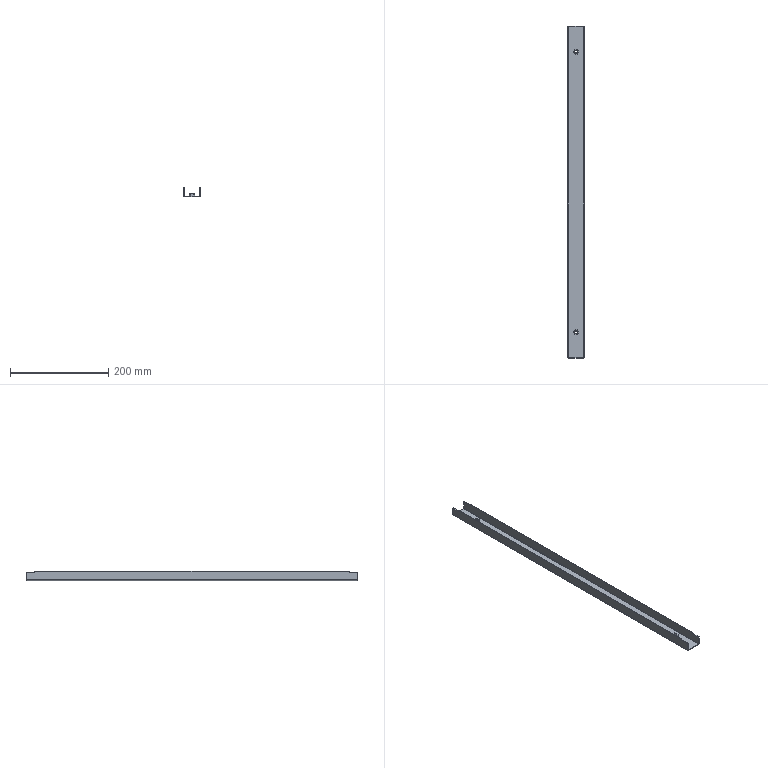Part | SolidWorks | features BaseBody 1 | 1 solid | 54 faces | box 33 x 674.5 x 20 mm | volume 70005 mm3 | plane 42 | cylinder 12 | commonest cylinder face diameters 6 x4 6.5 x4 1 x2 4 x2
STEP:
#1=CARTESIAN_POINT('',(3.,-285.,5.));
#2=VERTEX_POINT('',#1);
#3=CARTESIAN_POINT('',(3.,-285.,0.));
#4=VERTEX_POINT('',#3);
#5=CARTESIAN_POINT('',(3.,-285.,5.));
#6=DIRECTION('',(0.,0.,-1.));
#7=VECTOR('',#6,1000.);
#8=LINE('',#5,#7);
#9=EDGE_CURVE('',#2,#4,#8,.T.);
#10=ORIENTED_EDGE('',*,*,#9,.F.);
#11=CARTESIAN_POINT('',(-3.,-285.,5.));
#12=VERTEX_POINT('',#11);
#13=CARTESIAN_POINT('',(0.,-285.,5.));
#14=DIRECTION('',(0.,0.,1.));
#15=DIRECTION('',(1.,0.,0.));
#16=AXIS2_PLACEMENT_3D('',#13,#14,#15);
#17=CIRCLE('',#16,3.);
#18=EDGE_CURVE('',#2,#12,#17,.T.);
#19=ORIENTED_EDGE('',*,*,#18,.T.);
#20=CARTESIAN_POINT('',(-3.,-285.,0.));
#21=VERTEX_POINT('',#20);
#22=CARTESIAN_POINT('',(-3.,-285.,5.));
#23=DIRECTION('',(0.,0.,-1.));
#24=VECTOR('',#23,1000.);
#25=LINE('',#22,#24);
#26=EDGE_CURVE('',#12,#21,#25,.T.);
#27=ORIENTED_EDGE('',*,*,#26,.T.);
#28=CARTESIAN_POINT('',(0.,-285.,0.));
#29=DIRECTION('',(0.,0.,1.));
#30=DIRECTION('',(1.,0.,0.));
#31=AXIS2_PLACEMENT_3D('',#28,#29,#30);
#32=CIRCLE('',#31,3.);
#33=EDGE_CURVE('',#4,#21,#32,.T.);
#34=ORIENTED_EDGE('',*,*,#33,.F.);
#35=EDGE_LOOP('',(#10,#19,#27,#34));
#36=FACE_OUTER_BOUND('',#35,.T.);
#37=CARTESIAN_POINT('',(0.,-285.,5.));
#38=DIRECTION('',(0.,0.,-1.));
#39=DIRECTION('',(-1.,0.,0.));
#40=AXIS2_PLACEMENT_3D('',#37,#38,#39);
#41=CYLINDRICAL_SURFACE('',#40,3.);
#42=ADVANCED_FACE('',(#36),#41,.F.);
#43=CARTESIAN_POINT('',(3.629,-289.49,0.));
#44=VERTEX_POINT('',#43);
#45=CARTESIAN_POINT('',(5.703,-284.102,0.));
#46=VERTEX_POINT('',#45);
#47=CARTESIAN_POINT('',(3.629,-289.49,0.));
#48=DIRECTION('',(0.3592,0.9333,0.));
#49=VECTOR('',#48,1000.);
#50=LINE('',#47,#49);
#51=EDGE_CURVE('',#44,#46,#50,.T.);
#52=ORIENTED_EDGE('',*,*,#51,.T.);
#53=CARTESIAN_POINT('',(5.703,-284.102,5.));
#54=VERTEX_POINT('',#53);
#55=CARTESIAN_POINT('',(5.703,-284.102,5.));
#56=DIRECTION('',(0.,0.,-1.));
#57=VECTOR('',#56,1000.);
#58=LINE('',#55,#57);
#59=EDGE_CURVE('',#54,#46,#58,.T.);
#60=ORIENTED_EDGE('',*,*,#59,.F.);
#61=CARTESIAN_POINT('',(3.629,-289.49,5.));
#62=VERTEX_POINT('',#61);
#63=CARTESIAN_POINT('',(3.629,-289.49,5.));
#64=DIRECTION('',(0.3592,0.9333,0.));
#65=VECTOR('',#64,1000.);
#66=LINE('',#63,#65);
#67=EDGE_CURVE('',#62,#54,#66,.T.);
#68=ORIENTED_EDGE('',*,*,#67,.F.);
#69=CARTESIAN_POINT('',(3.629,-289.49,5.));
#70=DIRECTION('',(0.,0.,-1.));
#71=VECTOR('',#70,1000.);
#72=LINE('',#69,#71);
#73=EDGE_CURVE('',#62,#44,#72,.T.);
#74=ORIENTED_EDGE('',*,*,#73,.T.);
#75=EDGE_LOOP('',(#52,#60,#68,#74));
#76=FACE_OUTER_BOUND('',#75,.T.);
#77=CARTESIAN_POINT('',(3.629,-289.49,5.));
#78=DIRECTION('',(-0.9333,0.3592,0.));
#79=DIRECTION('',(0.,0.,1.));
#80=AXIS2_PLACEMENT_3D('',#77,#78,#79);
#81=PLANE('',#80);
#82=ADVANCED_FACE('',(#76),#81,.F.);
#83=CARTESIAN_POINT('',(-2.074,-290.388,0.));
#84=VERTEX_POINT('',#83);
#85=CARTESIAN_POINT('',(-2.074,-290.388,0.));
#86=DIRECTION('',(0.9878,0.1555,0.));
#87=VECTOR('',#86,1000.);
#88=LINE('',#85,#87);
#89=EDGE_CURVE('',#84,#44,#88,.T.);
#90=ORIENTED_EDGE('',*,*,#89,.T.);
#91=ORIENTED_EDGE('',*,*,#73,.F.);
#92=CARTESIAN_POINT('',(-2.074,-290.388,5.));
#93=VERTEX_POINT('',#92);
#94=CARTESIAN_POINT('',(-2.074,-290.388,5.));
#95=DIRECTION('',(0.9878,0.1555,0.));
#96=VECTOR('',#95,1000.);
#97=LINE('',#94,#96);
#98=EDGE_CURVE('',#93,#62,#97,.T.);
#99=ORIENTED_EDGE('',*,*,#98,.F.);
#100=CARTESIAN_POINT('',(-2.074,-290.388,5.));
#101=DIRECTION('',(0.,0.,-1.));
#102=VECTOR('',#101,1000.);
#103=LINE('',#100,#102);
#104=EDGE_CURVE('',#93,#84,#103,.T.);
#105=ORIENTED_EDGE('',*,*,#104,.T.);
#106=EDGE_LOOP('',(#90,#91,#99,#105));
#107=FACE_OUTER_BOUND('',#106,.T.);
#108=CARTESIAN_POINT('',(-2.074,-290.388,5.));
#109=DIRECTION('',(-0.1555,0.9878,0.));
#110=DIRECTION('',(0.,0.,1.));
#111=AXIS2_PLACEMENT_3D('',#108,#109,#110);
#112=PLANE('',#111);
#113=ADVANCED_FACE('',(#107),#112,.F.);
#114=CARTESIAN_POINT('',(-5.703,-285.898,0.));
#115=VERTEX_POINT('',#114);
#116=CARTESIAN_POINT('',(-5.703,-285.898,0.));
#117=DIRECTION('',(0.6286,-0.7777,0.));
#118=VECTOR('',#117,1000.);
#119=LINE('',#116,#118);
#120=EDGE_CURVE('',#115,#84,#119,.T.);
#121=ORIENTED_EDGE('',*,*,#120,.T.);
#122=ORIENTED_EDGE('',*,*,#104,.F.);
#123=CARTESIAN_POINT('',(-5.703,-285.898,5.));
#124=VERTEX_POINT('',#123);
#125=CARTESIAN_POINT('',(-5.703,-285.898,5.));
#126=DIRECTION('',(0.6286,-0.7777,0.));
#127=VECTOR('',#126,1000.);
#128=LINE('',#125,#127);
#129=EDGE_CURVE('',#124,#93,#128,.T.);
#130=ORIENTED_EDGE('',*,*,#129,.F.);
#131=CARTESIAN_POINT('',(-5.703,-285.898,5.));
#132=DIRECTION('',(0.,0.,-1.));
#133=VECTOR('',#132,1000.);
#134=LINE('',#131,#133);
#135=EDGE_CURVE('',#124,#115,#134,.T.);
#136=ORIENTED_EDGE('',*,*,#135,.T.);
#137=EDGE_LOOP('',(#121,#122,#130,#136));
#138=FACE_OUTER_BOUND('',#137,.T.);
#139=CARTESIAN_POINT('',(-5.703,-285.898,5.));
#140=DIRECTION('',(0.7777,0.6286,0.));
#141=DIRECTION('',(0.,0.,-1.));
#142=AXIS2_PLACEMENT_3D('',#139,#140,#141);
#143=PLANE('',#142);
#144=ADVANCED_FACE('',(#138),#143,.F.);
#145=CARTESIAN_POINT('',(-3.629,-280.51,0.));
#146=VERTEX_POINT('',#145);
#147=CARTESIAN_POINT('',(-3.629,-280.51,0.));
#148=DIRECTION('',(-0.3592,-0.9333,0.));
#149=VECTOR('',#148,1000.);
#150=LINE('',#147,#149);
#151=EDGE_CURVE('',#146,#115,#150,.T.);
#152=ORIENTED_EDGE('',*,*,#151,.T.);
#153=ORIENTED_EDGE('',*,*,#135,.F.);
#154=CARTESIAN_POINT('',(-3.629,-280.51,5.));
#155=VERTEX_POINT('',#154);
#156=CARTESIAN_POINT('',(-3.629,-280.51,5.));
#157=DIRECTION('',(-0.3592,-0.9333,0.));
#158=VECTOR('',#157,1000.);
#159=LINE('',#156,#158);
#160=EDGE_CURVE('',#155,#124,#159,.T.);
#161=ORIENTED_EDGE('',*,*,#160,.F.);
#162=CARTESIAN_POINT('',(-3.629,-280.51,5.));
#163=DIRECTION('',(0.,0.,-1.));
#164=VECTOR('',#163,1000.);
#165=LINE('',#162,#164);
#166=EDGE_CURVE('',#155,#146,#165,.T.);
#167=ORIENTED_EDGE('',*,*,#166,.T.);
#168=EDGE_LOOP('',(#152,#153,#161,#167));
#169=FACE_OUTER_BOUND('',#168,.T.);
#170=CARTESIAN_POINT('',(-3.629,-280.51,5.));
#171=DIRECTION('',(0.9333,-0.3592,0.));
#172=DIRECTION('',(0.,0.,-1.));
#173=AXIS2_PLACEMENT_3D('',#170,#171,#172);
#174=PLANE('',#173);
#175=ADVANCED_FACE('',(#169),#174,.F.);
#176=CARTESIAN_POINT('',(2.074,-279.612,0.));
#177=VERTEX_POINT('',#176);
#178=CARTESIAN_POINT('',(2.074,-279.612,0.));
#179=DIRECTION('',(-0.9878,-0.1555,0.));
#180=VECTOR('',#179,1000.);
#181=LINE('',#178,#180);
#182=EDGE_CURVE('',#177,#146,#181,.T.);
#183=ORIENTED_EDGE('',*,*,#182,.T.);
#184=ORIENTED_EDGE('',*,*,#166,.F.);
#185=CARTESIAN_POINT('',(2.074,-279.612,5.));
#186=VERTEX_POINT('',#185);
#187=CARTESIAN_POINT('',(2.074,-279.612,5.));
#188=DIRECTION('',(-0.9878,-0.1555,0.));
#189=VECTOR('',#188,1000.);
#190=LINE('',#187,#189);
#191=EDGE_CURVE('',#186,#155,#190,.T.);
#192=ORIENTED_EDGE('',*,*,#191,.F.);
#193=CARTESIAN_POINT('',(2.074,-279.612,5.));
#194=DIRECTION('',(0.,0.,-1.));
#195=VECTOR('',#194,1000.);
#196=LINE('',#193,#195);
#197=EDGE_CURVE('',#186,#177,#196,.T.);
#198=ORIENTED_EDGE('',*,*,#197,.T.);
#199=EDGE_LOOP('',(#183,#184,#192,#198));
#200=FACE_OUTER_BOUND('',#199,.T.);
#201=CARTESIAN_POINT('',(2.074,-279.612,5.));
#202=DIRECTION('',(0.1555,-0.9878,0.));
#203=DIRECTION('',(0.,0.,-1.));
#204=AXIS2_PLACEMENT_3D('',#201,#202,#203);
#205=PLANE('',#204);
#206=ADVANCED_FACE('',(#200),#205,.F.);
#207=CARTESIAN_POINT('',(5.703,-284.102,0.));
#208=DIRECTION('',(-0.6286,0.7777,0.));
#209=VECTOR('',#208,1000.);
#210=LINE('',#207,#209);
#211=EDGE_CURVE('',#46,#177,#210,.T.);
#212=ORIENTED_EDGE('',*,*,#211,.T.);
#213=ORIENTED_EDGE('',*,*,#197,.F.);
#214=CARTESIAN_POINT('',(5.703,-284.102,5.));
#215=DIRECTION('',(-0.6286,0.7777,0.));
#216=VECTOR('',#215,1000.);
#217=LINE('',#214,#216);
#218=EDGE_CURVE('',#54,#186,#217,.T.);
#219=ORIENTED_EDGE('',*,*,#218,.F.);
#220=ORIENTED_EDGE('',*,*,#59,.T.);
#221=EDGE_LOOP('',(#212,#213,#219,#220));
#222=FACE_OUTER_BOUND('',#221,.T.);
#223=CARTESIAN_POINT('',(5.703,-284.102,5.));
#224=DIRECTION('',(-0.7777,-0.6286,0.));
#225=DIRECTION('',(-0.6286,0.7777,0.));
#226=AXIS2_PLACEMENT_3D('',#223,#224,#225);
#227=PLANE('',#226);
#228=ADVANCED_FACE('',(#222),#227,.F.);
#229=CARTESIAN_POINT('',(0.,-285.,5.));
#230=DIRECTION('',(0.,0.,1.));
#231=DIRECTION('',(1.,0.,0.));
#232=AXIS2_PLACEMENT_3D('',#229,#230,#231);
#233=CIRCLE('',#232,3.);
#234=EDGE_CURVE('',#12,#2,#233,.T.);
#235=ORIENTED_EDGE('',*,*,#234,.F.);
#236=ORIENTED_EDGE('',*,*,#18,.F.);
#237=EDGE_LOOP('',(#235,#236));
#238=FACE_BOUND('',#237,.T.);
#239=ORIENTED_EDGE('',*,*,#218,.T.);
#240=ORIENTED_EDGE('',*,*,#191,.T.);
#241=ORIENTED_EDGE('',*,*,#160,.T.);
#242=ORIENTED_EDGE('',*,*,#129,.T.);
#243=ORIENTED_EDGE('',*,*,#98,.T.);
#244=ORIENTED_EDGE('',*,*,#67,.T.);
#245=EDGE_LOOP('',(#239,#240,#241,#242,#243,#244));
#246=FACE_OUTER_BOUND('',#245,.T.);
#247=CARTESIAN_POINT('',(0.,0.,5.));
#248=DIRECTION('',(0.,0.,1.));
#249=DIRECTION('',(1.,0.,0.));
#250=AXIS2_PLACEMENT_3D('',#247,#248,#249);
#251=PLANE('',#250);
#252=ADVANCED_FACE('',(#238,#246),#251,.T.);
#253=CARTESIAN_POINT('',(0.,-285.,0.));
#254=DIRECTION('',(0.,0.,1.));
#255=DIRECTION('',(1.,0.,0.));
#256=AXIS2_PLACEMENT_3D('',#253,#254,#255);
#257=CIRCLE('',#256,3.);
#258=EDGE_CURVE('',#21,#4,#257,.T.);
#259=ORIENTED_EDGE('',*,*,#258,.T.);
#260=ORIENTED_EDGE('',*,*,#33,.T.);
#261=EDGE_LOOP('',(#259,#260));
#262=FACE_BOUND('',#261,.T.);
#263=CARTESIAN_POINT('',(-3.25,-285.,0.));
#264=VERTEX_POINT('',#263);
#265=CARTESIAN_POINT('',(3.25,-285.,0.));
#266=VERTEX_POINT('',#265);
#267=CARTESIAN_POINT('',(0.,-285.,0.));
#268=DIRECTION('',(0.,0.,-1.));
#269=DIRECTION('',(-1.,0.,0.));
#270=AXIS2_PLACEMENT_3D('',#267,#268,#269);
#271=CIRCLE('',#270,3.25);
#272=EDGE_CURVE('',#264,#266,#271,.T.);
#273=ORIENTED_EDGE('',*,*,#272,.T.);
#274=CARTESIAN_POINT('',(0.,-285.,0.));
#275=DIRECTION('',(0.,0.,-1.));
#276=DIRECTION('',(-1.,0.,0.));
#277=AXIS2_PLACEMENT_3D('',#274,#275,#276);
#278=CIRCLE('',#277,3.25);
#279=EDGE_CURVE('',#266,#264,#278,.T.);
#280=ORIENTED_EDGE('',*,*,#279,.T.);
#281=EDGE_LOOP('',(#273,#280));
#282=FACE_OUTER_BOUND('',#281,.T.);
#283=CARTESIAN_POINT('',(0.,0.,0.));
#284=DIRECTION('',(0.,0.,1.));
#285=DIRECTION('',(1.,0.,0.));
#286=AXIS2_PLACEMENT_3D('',#283,#284,#285);
#287=PLANE('',#286);
#288=ADVANCED_FACE('',(#262,#282),#287,.F.);
#289=CARTESIAN_POINT('',(3.,285.,5.));
#290=VERTEX_POINT('',#289);
#291=CARTESIAN_POINT('',(3.,285.,0.));
#292=VERTEX_POINT('',#291);
#293=CARTESIAN_POINT('',(3.,285.,5.));
#294=DIRECTION('',(0.,0.,-1.));
#295=VECTOR('',#294,1000.);
#296=LINE('',#293,#295);
#297=EDGE_CURVE('',#290,#292,#296,.T.);
#298=ORIENTED_EDGE('',*,*,#297,.F.);
#299=CARTESIAN_POINT('',(-3.,285.,5.));
#300=VERTEX_POINT('',#299);
#301=CARTESIAN_POINT('',(0.,285.,5.));
#302=DIRECTION('',(0.,0.,1.));
#303=DIRECTION('',(1.,0.,0.));
#304=AXIS2_PLACEMENT_3D('',#301,#302,#303);
#305=CIRCLE('',#304,3.);
#306=EDGE_CURVE('',#290,#300,#305,.T.);
#307=ORIENTED_EDGE('',*,*,#306,.T.);
#308=CARTESIAN_POINT('',(-3.,285.,0.));
#309=VERTEX_POINT('',#308);
#310=CARTESIAN_POINT('',(-3.,285.,5.));
#311=DIRECTION('',(0.,0.,-1.));
#312=VECTOR('',#311,1000.);
#313=LINE('',#310,#312);
#314=EDGE_CURVE('',#300,#309,#313,.T.);
#315=ORIENTED_EDGE('',*,*,#314,.T.);
#316=CARTESIAN_POINT('',(0.,285.,0.));
#317=DIRECTION('',(0.,0.,1.));
#318=DIRECTION('',(1.,0.,0.));
#319=AXIS2_PLACEMENT_3D('',#316,#317,#318);
#320=CIRCLE('',#319,3.);
#321=EDGE_CURVE('',#292,#309,#320,.T.);
#322=ORIENTED_EDGE('',*,*,#321,.F.);
#323=EDGE_LOOP('',(#298,#307,#315,#322));
#324=FACE_OUTER_BOUND('',#323,.T.);
#325=CARTESIAN_POINT('',(0.,285.,5.));
#326=DIRECTION('',(0.,0.,-1.));
#327=DIRECTION('',(-1.,0.,0.));
#328=AXIS2_PLACEMENT_3D('',#325,#326,#327);
#329=CYLINDRICAL_SURFACE('',#328,3.);
#330=ADVANCED_FACE('',(#324),#329,.F.);
#331=CARTESIAN_POINT('',(-5.703,285.898,0.));
#332=VERTEX_POINT('',#331);
#333=CARTESIAN_POINT('',(-3.629,280.51,0.));
#334=VERTEX_POINT('',#333);
#335=CARTESIAN_POINT('',(-5.703,285.898,0.));
#336=DIRECTION('',(0.3592,-0.9333,0.));
#337=VECTOR('',#336,1000.);
#338=LINE('',#335,#337);
#339=EDGE_CURVE('',#332,#334,#338,.T.);
#340=ORIENTED_EDGE('',*,*,#339,.T.);
#341=CARTESIAN_POINT('',(-3.629,280.51,5.));
#342=VERTEX_POINT('',#341);
#343=CARTESIAN_POINT('',(-3.629,280.51,5.));
#344=DIRECTION('',(0.,0.,-1.));
#345=VECTOR('',#344,1000.);
#346=LINE('',#343,#345);
#347=EDGE_CURVE('',#342,#334,#346,.T.);
#348=ORIENTED_EDGE('',*,*,#347,.F.);
#349=CARTESIAN_POINT('',(-5.703,285.898,5.));
#350=VERTEX_POINT('',#349);
#351=CARTESIAN_POINT('',(-5.703,285.898,5.));
#352=DIRECTION('',(0.3592,-0.9333,0.));
#353=VECTOR('',#352,1000.);
#354=LINE('',#351,#353);
#355=EDGE_CURVE('',#350,#342,#354,.T.);
#356=ORIENTED_EDGE('',*,*,#355,.F.);
#357=CARTESIAN_POINT('',(-5.703,285.898,5.));
#358=DIRECTION('',(0.,0.,-1.));
#359=VECTOR('',#358,1000.);
#360=LINE('',#357,#359);
#361=EDGE_CURVE('',#350,#332,#360,.T.);
#362=ORIENTED_EDGE('',*,*,#361,.T.);
#363=EDGE_LOOP('',(#340,#348,#356,#362));
#364=FACE_OUTER_BOUND('',#363,.T.);
#365=CARTESIAN_POINT('',(-5.703,285.898,5.));
#366=DIRECTION('',(0.9333,0.3592,0.));
#367=DIRECTION('',(0.,0.,-1.));
#368=AXIS2_PLACEMENT_3D('',#365,#366,#367);
#369=PLANE('',#368);
#370=ADVANCED_FACE('',(#364),#369,.F.);
#371=CARTESIAN_POINT('',(-2.074,290.388,0.));
#372=VERTEX_POINT('',#371);
#373=CARTESIAN_POINT('',(-2.074,290.388,0.));
#374=DIRECTION('',(-0.6286,-0.7777,0.));
#375=VECTOR('',#374,1000.);
#376=LINE('',#373,#375);
#377=EDGE_CURVE('',#372,#332,#376,.T.);
#378=ORIENTED_EDGE('',*,*,#377,.T.);
#379=ORIENTED_EDGE('',*,*,#361,.F.);
#380=CARTESIAN_POINT('',(-2.074,290.388,5.));
#381=VERTEX_POINT('',#380);
#382=CARTESIAN_POINT('',(-2.074,290.388,5.));
#383=DIRECTION('',(-0.6286,-0.7777,0.));
#384=VECTOR('',#383,1000.);
#385=LINE('',#382,#384);
#386=EDGE_CURVE('',#381,#350,#385,.T.);
#387=ORIENTED_EDGE('',*,*,#386,.F.);
#388=CARTESIAN_POINT('',(-2.074,290.388,5.));
#389=DIRECTION('',(0.,0.,-1.));
#390=VECTOR('',#389,1000.);
#391=LINE('',#388,#390);
#392=EDGE_CURVE('',#381,#372,#391,.T.);
#393=ORIENTED_EDGE('',*,*,#392,.T.);
#394=EDGE_LOOP('',(#378,#379,#387,#393));
#395=FACE_OUTER_BOUND('',#394,.T.);
#396=CARTESIAN_POINT('',(-2.074,290.388,5.));
#397=DIRECTION('',(0.7777,-0.6286,0.));
#398=DIRECTION('',(0.,0.,-1.));
#399=AXIS2_PLACEMENT_3D('',#396,#397,#398);
#400=PLANE('',#399);
#401=ADVANCED_FACE('',(#395),#400,.F.);
#402=CARTESIAN_POINT('',(3.629,289.49,0.));
#403=VERTEX_POINT('',#402);
#404=CARTESIAN_POINT('',(3.629,289.49,0.));
#405=DIRECTION('',(-0.9878,0.1555,0.));
#406=VECTOR('',#405,1000.);
#407=LINE('',#404,#406);
#408=EDGE_CURVE('',#403,#372,#407,.T.);
#409=ORIENTED_EDGE('',*,*,#408,.T.);
#410=ORIENTED_EDGE('',*,*,#392,.F.);
#411=CARTESIAN_POINT('',(3.629,289.49,5.));
#412=VERTEX_POINT('',#411);
#413=CARTESIAN_POINT('',(3.629,289.49,5.));
#414=DIRECTION('',(-0.9878,0.1555,0.));
#415=VECTOR('',#414,1000.);
#416=LINE('',#413,#415);
#417=EDGE_CURVE('',#412,#381,#416,.T.);
#418=ORIENTED_EDGE('',*,*,#417,.F.);
#419=CARTESIAN_POINT('',(3.629,289.49,5.));
#420=DIRECTION('',(0.,0.,-1.));
#421=VECTOR('',#420,1000.);
#422=LINE('',#419,#421);
#423=EDGE_CURVE('',#412,#403,#422,.T.);
#424=ORIENTED_EDGE('',*,*,#423,.T.);
#425=EDGE_LOOP('',(#409,#410,#418,#424));
#426=FACE_OUTER_BOUND('',#425,.T.);
#427=CARTESIAN_POINT('',(3.629,289.49,5.));
#428=DIRECTION('',(-0.1555,-0.9878,0.));
#429=DIRECTION('',(-0.9878,0.1555,0.));
#430=AXIS2_PLACEMENT_3D('',#427,#428,#429);
#431=PLANE('',#430);
#432=ADVANCED_FACE('',(#426),#431,.F.);
#433=CARTESIAN_POINT('',(5.703,284.102,0.));
#434=VERTEX_POINT('',#433);
#435=CARTESIAN_POINT('',(5.703,284.102,0.));
#436=DIRECTION('',(-0.3592,0.9333,0.));
#437=VECTOR('',#436,1000.);
#438=LINE('',#435,#437);
#439=EDGE_CURVE('',#434,#403,#438,.T.);
#440=ORIENTED_EDGE('',*,*,#439,.T.);
#441=ORIENTED_EDGE('',*,*,#423,.F.);
#442=CARTESIAN_POINT('',(5.703,284.102,5.));
#443=VERTEX_POINT('',#442);
#444=CARTESIAN_POINT('',(5.703,284.102,5.));
#445=DIRECTION('',(-0.3592,0.9333,0.));
#446=VECTOR('',#445,1000.);
#447=LINE('',#444,#446);
#448=EDGE_CURVE('',#443,#412,#447,.T.);
#449=ORIENTED_EDGE('',*,*,#448,.F.);
#450=CARTESIAN_POINT('',(5.703,284.102,5.));
#451=DIRECTION('',(0.,0.,-1.));
#452=VECTOR('',#451,1000.);
#453=LINE('',#450,#452);
#454=EDGE_CURVE('',#443,#434,#453,.T.);
#455=ORIENTED_EDGE('',*,*,#454,.T.);
#456=EDGE_LOOP('',(#440,#441,#449,#455));
#457=FACE_OUTER_BOUND('',#456,.T.);
#458=CARTESIAN_POINT('',(5.703,284.102,5.));
#459=DIRECTION('',(-0.9333,-0.3592,0.));
#460=DIRECTION('',(-0.3592,0.9333,0.));
#461=AXIS2_PLACEMENT_3D('',#458,#459,#460);
#462=PLANE('',#461);
#463=ADVANCED_FACE('',(#457),#462,.F.);
#464=CARTESIAN_POINT('',(2.074,279.612,0.));
#465=VERTEX_POINT('',#464);
#466=CARTESIAN_POINT('',(2.074,279.612,0.));
#467=DIRECTION('',(0.6286,0.7777,0.));
#468=VECTOR('',#467,1000.);
#469=LINE('',#466,#468);
#470=EDGE_CURVE('',#465,#434,#469,.T.);
#471=ORIENTED_EDGE('',*,*,#470,.T.);
#472=ORIENTED_EDGE('',*,*,#454,.F.);
#473=CARTESIAN_POINT('',(2.074,279.612,5.));
#474=VERTEX_POINT('',#473);
#475=CARTESIAN_POINT('',(2.074,279.612,5.));
#476=DIRECTION('',(0.6286,0.7777,0.));
#477=VECTOR('',#476,1000.);
#478=LINE('',#475,#477);
#479=EDGE_CURVE('',#474,#443,#478,.T.);
#480=ORIENTED_EDGE('',*,*,#479,.F.);
#481=CARTESIAN_POINT('',(2.074,279.612,5.));
#482=DIRECTION('',(0.,0.,-1.));
#483=VECTOR('',#482,1000.);
#484=LINE('',#481,#483);
#485=EDGE_CURVE('',#474,#465,#484,.T.);
#486=ORIENTED_EDGE('',*,*,#485,.T.);
#487=EDGE_LOOP('',(#471,#472,#480,#486));
#488=FACE_OUTER_BOUND('',#487,.T.);
#489=CARTESIAN_POINT('',(2.074,279.612,5.));
#490=DIRECTION('',(-0.7777,0.6286,0.));
#491=DIRECTION('',(0.,0.,1.));
#492=AXIS2_PLACEMENT_3D('',#489,#490,#491);
#493=PLANE('',#492);
#494=ADVANCED_FACE('',(#488),#493,.F.);
#495=CARTESIAN_POINT('',(-3.629,280.51,0.));
#496=DIRECTION('',(0.9878,-0.1555,0.));
#497=VECTOR('',#496,1000.);
#498=LINE('',#495,#497);
#499=EDGE_CURVE('',#334,#465,#498,.T.);
#500=ORIENTED_EDGE('',*,*,#499,.T.);
#501=ORIENTED_EDGE('',*,*,#485,.F.);
#502=CARTESIAN_POINT('',(-3.629,280.51,5.));
#503=DIRECTION('',(0.9878,-0.1555,0.));
#504=VECTOR('',#503,1000.);
#505=LINE('',#502,#504);
#506=EDGE_CURVE('',#342,#474,#505,.T.);
#507=ORIENTED_EDGE('',*,*,#506,.F.);
#508=ORIENTED_EDGE('',*,*,#347,.T.);
#509=EDGE_LOOP('',(#500,#501,#507,#508));
#510=FACE_OUTER_BOUND('',#509,.T.);
#511=CARTESIAN_POINT('',(-3.629,280.51,5.));
#512=DIRECTION('',(0.1555,0.9878,0.));
#513=DIRECTION('',(0.,0.,-1.));
#514=AXIS2_PLACEMENT_3D('',#511,#512,#513);
#515=PLANE('',#514);
#516=ADVANCED_FACE('',(#510),#515,.F.);
#517=CARTESIAN_POINT('',(0.,285.,5.));
#518=DIRECTION('',(0.,0.,1.));
#519=DIRECTION('',(1.,0.,0.));
#520=AXIS2_PLACEMENT_3D('',#517,#518,#519);
#521=CIRCLE('',#520,3.);
#522=EDGE_CURVE('',#300,#290,#521,.T.);
#523=ORIENTED_EDGE('',*,*,#522,.F.);
#524=ORIENTED_EDGE('',*,*,#306,.F.);
#525=EDGE_LOOP('',(#523,#524));
#526=FACE_BOUND('',#525,.T.);
#527=ORIENTED_EDGE('',*,*,#506,.T.);
#528=ORIENTED_EDGE('',*,*,#479,.T.);
#529=ORIENTED_EDGE('',*,*,#448,.T.);
#530=ORIENTED_EDGE('',*,*,#417,.T.);
#531=ORIENTED_EDGE('',*,*,#386,.T.);
#532=ORIENTED_EDGE('',*,*,#355,.T.);
#533=EDGE_LOOP('',(#527,#528,#529,#530,#531,#532));
#534=FACE_OUTER_BOUND('',#533,.T.);
#535=CARTESIAN_POINT('',(0.,0.,5.));
#536=DIRECTION('',(0.,0.,1.));
#537=DIRECTION('',(1.,0.,0.));
#538=AXIS2_PLACEMENT_3D('',#535,#536,#537);
#539=PLANE('',#538);
#540=ADVANCED_FACE('',(#526,#534),#539,.T.);
#541=CARTESIAN_POINT('',(0.,285.,0.));
#542=DIRECTION('',(0.,0.,1.));
#543=DIRECTION('',(1.,0.,0.));
#544=AXIS2_PLACEMENT_3D('',#541,#542,#543);
#545=CIRCLE('',#544,3.);
#546=EDGE_CURVE('',#309,#292,#545,.T.);
#547=ORIENTED_EDGE('',*,*,#546,.T.);
#548=ORIENTED_EDGE('',*,*,#321,.T.);
#549=EDGE_LOOP('',(#547,#548));
#550=FACE_BOUND('',#549,.T.);
#551=CARTESIAN_POINT('',(-3.25,285.,0.));
#552=VERTEX_POINT('',#551);
#553=CARTESIAN_POINT('',(3.25,285.,0.));
#554=VERTEX_POINT('',#553);
#555=CARTESIAN_POINT('',(0.,285.,0.));
#556=DIRECTION('',(0.,0.,-1.));
#557=DIRECTION('',(-1.,0.,0.));
#558=AXIS2_PLACEMENT_3D('',#555,#556,#557);
#559=CIRCLE('',#558,3.25);
#560=EDGE_CURVE('',#552,#554,#559,.T.);
#561=ORIENTED_EDGE('',*,*,#560,.T.);
#562=CARTESIAN_POINT('',(0.,285.,0.));
#563=DIRECTION('',(0.,0.,-1.));
#564=DIRECTION('',(-1.,0.,0.));
#565=AXIS2_PLACEMENT_3D('',#562,#563,#564);
#566=CIRCLE('',#565,3.25);
#567=EDGE_CURVE('',#554,#552,#566,.T.);
#568=ORIENTED_EDGE('',*,*,#567,.T.);
#569=EDGE_LOOP('',(#561,#568));
#570=FACE_OUTER_BOUND('',#569,.T.);
#571=CARTESIAN_POINT('',(0.,0.,0.));
#572=DIRECTION('',(0.,0.,1.));
#573=DIRECTION('',(1.,0.,0.));
#574=AXIS2_PLACEMENT_3D('',#571,#572,#573);
#575=PLANE('',#574);
#576=ADVANCED_FACE('',(#550,#570),#575,.F.);
#577=CARTESIAN_POINT('',(-15.,319.25,18.5));
#578=VERTEX_POINT('',#577);
#579=CARTESIAN_POINT('',(-15.,319.25,16.5));
#580=VERTEX_POINT('',#579);
#581=CARTESIAN_POINT('',(-15.,319.25,0.));
#582=DIRECTION('',(0.,0.,-1.));
#583=VECTOR('',#582,1000.);
#584=LINE('',#581,#583);
#585=EDGE_CURVE('',#578,#580,#584,.T.);
#586=ORIENTED_EDGE('',*,*,#585,.T.);
#587=CARTESIAN_POINT('',(-16.5,319.25,16.5));
#588=VERTEX_POINT('',#587);
#589=CARTESIAN_POINT('',(-16.5,319.25,16.5));
#590=DIRECTION('',(1.,0.,0.));
#591=VECTOR('',#590,1000.);
#592=LINE('',#589,#591);
#593=EDGE_CURVE('',#588,#580,#592,.T.);
#594=ORIENTED_EDGE('',*,*,#593,.F.);
#595=CARTESIAN_POINT('',(-16.5,319.25,18.5));
#596=VERTEX_POINT('',#595);
#597=CARTESIAN_POINT('',(-16.5,319.25,18.5));
#598=DIRECTION('',(0.,0.,-1.));
#599=VECTOR('',#598,1000.);
#600=LINE('',#597,#599);
#601=EDGE_CURVE('',#596,#588,#600,.T.);
#602=ORIENTED_EDGE('',*,*,#601,.F.);
#603=CARTESIAN_POINT('',(-16.5,319.25,18.5));
#604=DIRECTION('',(1.,0.,0.));
#605=VECTOR('',#604,1000.);
#606=LINE('',#603,#605);
#607=EDGE_CURVE('',#596,#578,#606,.T.);
#608=ORIENTED_EDGE('',*,*,#607,.T.);
#609=EDGE_LOOP('',(#586,#594,#602,#608));
#610=FACE_OUTER_BOUND('',#609,.T.);
#611=CARTESIAN_POINT('',(-16.5,319.25,18.5));
#612=DIRECTION('',(0.,-1.,0.));
#613=DIRECTION('',(0.,0.,-1.));
#614=AXIS2_PLACEMENT_3D('',#611,#612,#613);
#615=PLANE('',#614);
#616=ADVANCED_FACE('',(#610),#615,.F.);
#617=CARTESIAN_POINT('',(-15.,337.25,16.5));
#618=VERTEX_POINT('',#617);
#619=CARTESIAN_POINT('',(-15.,0.,16.5));
#620=DIRECTION('',(0.,1.,0.));
#621=VECTOR('',#620,1000.);
#622=LINE('',#619,#621);
#623=EDGE_CURVE('',#580,#618,#622,.T.);
#624=ORIENTED_EDGE('',*,*,#623,.T.);
#625=CARTESIAN_POINT('',(-16.5,337.25,16.5));
#626=VERTEX_POINT('',#625);
#627=CARTESIAN_POINT('',(-16.5,337.25,16.5));
#628=DIRECTION('',(1.,0.,0.));
#629=VECTOR('',#628,1000.);
#630=LINE('',#627,#629);
#631=EDGE_CURVE('',#626,#618,#630,.T.);
#632=ORIENTED_EDGE('',*,*,#631,.F.);
#633=CARTESIAN_POINT('',(-16.5,337.25,16.5));
#634=DIRECTION('',(0.,1.,0.));
#635=VECTOR('',#634,1000.);
#636=LINE('',#633,#635);
#637=EDGE_CURVE('',#588,#626,#636,.T.);
#638=ORIENTED_EDGE('',*,*,#637,.F.);
#639=ORIENTED_EDGE('',*,*,#593,.T.);
#640=EDGE_LOOP('',(#624,#632,#638,#639));
#641=FACE_OUTER_BOUND('',#640,.T.);
#642=CARTESIAN_POINT('',(-16.5,337.25,16.5));
#643=DIRECTION('',(0.,0.,-1.));
#644=DIRECTION('',(-1.,0.,0.));
#645=AXIS2_PLACEMENT_3D('',#642,#643,#644);
#646=PLANE('',#645);
#647=ADVANCED_FACE('',(#641),#646,.F.);
#648=CARTESIAN_POINT('',(-15.,-319.25,16.5));
#649=VERTEX_POINT('',#648);
#650=CARTESIAN_POINT('',(-15.,-319.25,18.5));
#651=VERTEX_POINT('',#650);
#652=CARTESIAN_POINT('',(-15.,-319.25,0.));
#653=DIRECTION('',(0.,0.,1.));
#654=VECTOR('',#653,1000.);
#655=LINE('',#652,#654);
#656=EDGE_CURVE('',#649,#651,#655,.T.);
#657=ORIENTED_EDGE('',*,*,#656,.T.);
#658=CARTESIAN_POINT('',(-16.5,-319.25,18.5));
#659=VERTEX_POINT('',#658);
#660=CARTESIAN_POINT('',(-16.5,-319.25,18.5));
#661=DIRECTION('',(1.,0.,0.));
#662=VECTOR('',#661,1000.);
#663=LINE('',#660,#662);
#664=EDGE_CURVE('',#659,#651,#663,.T.);
#665=ORIENTED_EDGE('',*,*,#664,.F.);
#666=CARTESIAN_POINT('',(-16.5,-319.25,16.5));
#667=VERTEX_POINT('',#666);
#668=CARTESIAN_POINT('',(-16.5,-319.25,18.5));
#669=DIRECTION('',(0.,0.,1.));
#670=VECTOR('',#669,1000.);
#671=LINE('',#668,#670);
#672=EDGE_CURVE('',#667,#659,#671,.T.);
#673=ORIENTED_EDGE('',*,*,#672,.F.);
#674=CARTESIAN_POINT('',(-16.5,-319.25,16.5));
#675=DIRECTION('',(1.,0.,0.));
#676=VECTOR('',#675,1000.);
#677=LINE('',#674,#676);
#678=EDGE_CURVE('',#667,#649,#677,.T.);
#679=ORIENTED_EDGE('',*,*,#678,.T.);
#680=EDGE_LOOP('',(#657,#665,#673,#679));
#681=FACE_OUTER_BOUND('',#680,.T.);
#682=CARTESIAN_POINT('',(-16.5,-319.25,18.5));
#683=DIRECTION('',(0.,1.,0.));
#684=DIRECTION('',(1.,0.,0.));
#685=AXIS2_PLACEMENT_3D('',#682,#683,#684);
#686=PLANE('',#685);
#687=ADVANCED_FACE('',(#681),#686,.F.);
#688=CARTESIAN_POINT('',(-15.,-337.25,16.5));
#689=VERTEX_POINT('',#688);
#690=CARTESIAN_POINT('',(-15.,0.,16.5));
#691=DIRECTION('',(0.,1.,0.));
#692=VECTOR('',#691,1000.);
#693=LINE('',#690,#692);
#694=EDGE_CURVE('',#689,#649,#693,.T.);
#695=ORIENTED_EDGE('',*,*,#694,.T.);
#696=ORIENTED_EDGE('',*,*,#678,.F.);
#697=CARTESIAN_POINT('',(-16.5,-337.25,16.5));
#698=VERTEX_POINT('',#697);
#699=CARTESIAN_POINT('',(-16.5,-337.25,16.5));
#700=DIRECTION('',(0.,1.,0.));
#701=VECTOR('',#700,1000.);
#702=LINE('',#699,#701);
#703=EDGE_CURVE('',#698,#667,#702,.T.);
#704=ORIENTED_EDGE('',*,*,#703,.F.);
#705=CARTESIAN_POINT('',(-16.5,-337.25,16.5));
#706=DIRECTION('',(1.,0.,0.));
#707=VECTOR('',#706,1000.);
#708=LINE('',#705,#707);
#709=EDGE_CURVE('',#698,#689,#708,.T.);
#710=ORIENTED_EDGE('',*,*,#709,.T.);
#711=EDGE_LOOP('',(#695,#696,#704,#710));
#712=FACE_OUTER_BOUND('',#711,.T.);
#713=CARTESIAN_POINT('',(-16.5,-337.25,16.5));
#714=DIRECTION('',(0.,0.,-1.));
#715=DIRECTION('',(-1.,0.,0.));
#716=AXIS2_PLACEMENT_3D('',#713,#714,#715);
#717=PLANE('',#716);
#718=ADVANCED_FACE('',(#712),#717,.F.);
#719=CARTESIAN_POINT('',(15.,337.25,16.5));
#720=VERTEX_POINT('',#719);
#721=CARTESIAN_POINT('',(15.,319.25,16.5));
#722=VERTEX_POINT('',#721);
#723=CARTESIAN_POINT('',(15.,0.,16.5));
#724=DIRECTION('',(0.,-1.,0.));
#725=VECTOR('',#724,1000.);
#726=LINE('',#723,#725);
#727=EDGE_CURVE('',#720,#722,#726,.T.);
#728=ORIENTED_EDGE('',*,*,#727,.T.);
#729=CARTESIAN_POINT('',(16.5,319.25,16.5));
#730=VERTEX_POINT('',#729);
#731=CARTESIAN_POINT('',(-16.5,319.25,16.5));
#732=DIRECTION('',(1.,0.,0.));
#733=VECTOR('',#732,1000.);
#734=LINE('',#731,#733);
#735=EDGE_CURVE('',#722,#730,#734,.T.);
#736=ORIENTED_EDGE('',*,*,#735,.T.);
#737=CARTESIAN_POINT('',(16.5,337.25,16.5));
#738=VERTEX_POINT('',#737);
#739=CARTESIAN_POINT('',(16.5,337.25,16.5));
#740=DIRECTION('',(0.,1.,0.));
#741=VECTOR('',#740,1000.);
#742=LINE('',#739,#741);
#743=EDGE_CURVE('',#730,#738,#742,.T.);
#744=ORIENTED_EDGE('',*,*,#743,.T.);
#745=CARTESIAN_POINT('',(-16.5,337.25,16.5));
#746=DIRECTION('',(1.,0.,0.));
#747=VECTOR('',#746,1000.);
#748=LINE('',#745,#747);
#749=EDGE_CURVE('',#720,#738,#748,.T.);
#750=ORIENTED_EDGE('',*,*,#749,.F.);
#751=EDGE_LOOP('',(#728,#736,#744,#750));
#752=FACE_OUTER_BOUND('',#751,.T.);
#753=CARTESIAN_POINT('',(-16.5,337.25,16.5));
#754=DIRECTION('',(0.,0.,-1.));
#755=DIRECTION('',(-1.,0.,0.));
#756=AXIS2_PLACEMENT_3D('',#753,#754,#755);
#757=PLANE('',#756);
#758=ADVANCED_FACE('',(#752),#757,.F.);
#759=CARTESIAN_POINT('',(15.,319.25,18.5));
#760=VERTEX_POINT('',#759);
#761=CARTESIAN_POINT('',(15.,319.25,0.));
#762=DIRECTION('',(0.,0.,1.));
#763=VECTOR('',#762,1000.);
#764=LINE('',#761,#763);
#765=EDGE_CURVE('',#722,#760,#764,.T.);
#766=ORIENTED_EDGE('',*,*,#765,.T.);
#767=CARTESIAN_POINT('',(16.5,319.25,18.5));
#768=VERTEX_POINT('',#767);
#769=CARTESIAN_POINT('',(16.5,319.25,18.5));
#770=DIRECTION('',(-1.,0.,0.));
#771=VECTOR('',#770,1000.);
#772=LINE('',#769,#771);
#773=EDGE_CURVE('',#768,#760,#772,.T.);
#774=ORIENTED_EDGE('',*,*,#773,.F.);
#775=CARTESIAN_POINT('',(16.5,319.25,18.5));
#776=DIRECTION('',(0.,0.,-1.));
#777=VECTOR('',#776,1000.);
#778=LINE('',#775,#777);
#779=EDGE_CURVE('',#768,#730,#778,.T.);
#780=ORIENTED_EDGE('',*,*,#779,.T.);
#781=ORIENTED_EDGE('',*,*,#735,.F.);
#782=EDGE_LOOP('',(#766,#774,#780,#781));
#783=FACE_OUTER_BOUND('',#782,.T.);
#784=CARTESIAN_POINT('',(-16.5,319.25,18.5));
#785=DIRECTION('',(0.,-1.,0.));
#786=DIRECTION('',(0.,0.,-1.));
#787=AXIS2_PLACEMENT_3D('',#784,#785,#786);
#788=PLANE('',#787);
#789=ADVANCED_FACE('',(#783),#788,.F.);
#790=CARTESIAN_POINT('',(15.,-319.25,16.5));
#791=VERTEX_POINT('',#790);
#792=CARTESIAN_POINT('',(15.,-337.25,16.5));
#793=VERTEX_POINT('',#792);
#794=CARTESIAN_POINT('',(15.,0.,16.5));
#795=DIRECTION('',(0.,-1.,0.));
#796=VECTOR('',#795,1000.);
#797=LINE('',#794,#796);
#798=EDGE_CURVE('',#791,#793,#797,.T.);
#799=ORIENTED_EDGE('',*,*,#798,.T.);
#800=CARTESIAN_POINT('',(16.5,-337.25,16.5));
#801=VERTEX_POINT('',#800);
#802=CARTESIAN_POINT('',(-16.5,-337.25,16.5));
#803=DIRECTION('',(1.,0.,0.));
#804=VECTOR('',#803,1000.);
#805=LINE('',#802,#804);
#806=EDGE_CURVE('',#793,#801,#805,.T.);
#807=ORIENTED_EDGE('',*,*,#806,.T.);
#808=CARTESIAN_POINT('',(16.5,-319.25,16.5));
#809=VERTEX_POINT('',#808);
#810=CARTESIAN_POINT('',(16.5,-337.25,16.5));
#811=DIRECTION('',(0.,1.,0.));
#812=VECTOR('',#811,1000.);
#813=LINE('',#810,#812);
#814=EDGE_CURVE('',#801,#809,#813,.T.);
#815=ORIENTED_EDGE('',*,*,#814,.T.);
#816=CARTESIAN_POINT('',(-16.5,-319.25,16.5));
#817=DIRECTION('',(1.,0.,0.));
#818=VECTOR('',#817,1000.);
#819=LINE('',#816,#818);
#820=EDGE_CURVE('',#791,#809,#819,.T.);
#821=ORIENTED_EDGE('',*,*,#820,.F.);
#822=EDGE_LOOP('',(#799,#807,#815,#821));
#823=FACE_OUTER_BOUND('',#822,.T.);
#824=CARTESIAN_POINT('',(-16.5,-337.25,16.5));
#825=DIRECTION('',(0.,0.,-1.));
#826=DIRECTION('',(-1.,0.,0.));
#827=AXIS2_PLACEMENT_3D('',#824,#825,#826);
#828=PLANE('',#827);
#829=ADVANCED_FACE('',(#823),#828,.F.);
#830=CARTESIAN_POINT('',(15.,-319.25,18.5));
#831=VERTEX_POINT('',#830);
#832=CARTESIAN_POINT('',(15.,-319.25,0.));
#833=DIRECTION('',(0.,0.,-1.));
#834=VECTOR('',#833,1000.);
#835=LINE('',#832,#834);
#836=EDGE_CURVE('',#831,#791,#835,.T.);
#837=ORIENTED_EDGE('',*,*,#836,.T.);
#838=ORIENTED_EDGE('',*,*,#820,.T.);
#839=CARTESIAN_POINT('',(16.5,-319.25,18.5));
#840=VERTEX_POINT('',#839);
#841=CARTESIAN_POINT('',(16.5,-319.25,18.5));
#842=DIRECTION('',(0.,0.,1.));
#843=VECTOR('',#842,1000.);
#844=LINE('',#841,#843);
#845=EDGE_CURVE('',#809,#840,#844,.T.);
#846=ORIENTED_EDGE('',*,*,#845,.T.);
#847=CARTESIAN_POINT('',(16.5,-319.25,18.5));
#848=DIRECTION('',(1.,0.,0.));
#849=VECTOR('',#848,1000.);
#850=LINE('',#847,#849);
#851=EDGE_CURVE('',#831,#840,#850,.T.);
#852=ORIENTED_EDGE('',*,*,#851,.F.);
#853=EDGE_LOOP('',(#837,#838,#846,#852));
#854=FACE_OUTER_BOUND('',#853,.T.);
#855=CARTESIAN_POINT('',(-16.5,-319.25,18.5));
#856=DIRECTION('',(0.,1.,0.));
#857=DIRECTION('',(1.,0.,0.));
#858=AXIS2_PLACEMENT_3D('',#855,#856,#857);
#859=PLANE('',#858);
#860=ADVANCED_FACE('',(#854),#859,.F.);
#861=CARTESIAN_POINT('',(3.25,285.,-1.5));
#862=VERTEX_POINT('',#861);
#863=CARTESIAN_POINT('',(3.25,285.,0.));
#864=DIRECTION('',(0.,0.,-1.));
#865=VECTOR('',#864,1000.);
#866=LINE('',#863,#865);
#867=EDGE_CURVE('',#554,#862,#866,.T.);
#868=ORIENTED_EDGE('',*,*,#867,.F.);
#869=ORIENTED_EDGE('',*,*,#560,.F.);
#870=CARTESIAN_POINT('',(-3.25,285.,-1.5));
#871=VERTEX_POINT('',#870);
#872=CARTESIAN_POINT('',(-3.25,285.,0.));
#873=DIRECTION('',(0.,0.,-1.));
#874=VECTOR('',#873,1000.);
#875=LINE('',#872,#874);
#876=EDGE_CURVE('',#552,#871,#875,.T.);
#877=ORIENTED_EDGE('',*,*,#876,.T.);
#878=CARTESIAN_POINT('',(0.,285.,-1.5));
#879=DIRECTION('',(0.,0.,-1.));
#880=DIRECTION('',(-1.,0.,0.));
#881=AXIS2_PLACEMENT_3D('',#878,#879,#880);
#882=CIRCLE('',#881,3.25);
#883=EDGE_CURVE('',#871,#862,#882,.T.);
#884=ORIENTED_EDGE('',*,*,#883,.T.);
#885=EDGE_LOOP('',(#868,#869,#877,#884));
#886=FACE_OUTER_BOUND('',#885,.T.);
#887=CARTESIAN_POINT('',(0.,285.,0.));
#888=DIRECTION('',(0.,0.,-1.));
#889=DIRECTION('',(-1.,0.,0.));
#890=AXIS2_PLACEMENT_3D('',#887,#888,#889);
#891=CYLINDRICAL_SURFACE('',#890,3.25);
#892=ADVANCED_FACE('',(#886),#891,.F.);
#893=CARTESIAN_POINT('',(3.25,-285.,-1.5));
#894=VERTEX_POINT('',#893);
#895=CARTESIAN_POINT('',(3.25,-285.,0.));
#896=DIRECTION('',(0.,0.,-1.));
#897=VECTOR('',#896,1000.);
#898=LINE('',#895,#897);
#899=EDGE_CURVE('',#266,#894,#898,.T.);
#900=ORIENTED_EDGE('',*,*,#899,.F.);
#901=ORIENTED_EDGE('',*,*,#272,.F.);
#902=CARTESIAN_POINT('',(-3.25,-285.,-1.5));
#903=VERTEX_POINT('',#902);
#904=CARTESIAN_POINT('',(-3.25,-285.,0.));
#905=DIRECTION('',(0.,0.,-1.));
#906=VECTOR('',#905,1000.);
#907=LINE('',#904,#906);
#908=EDGE_CURVE('',#264,#903,#907,.T.);
#909=ORIENTED_EDGE('',*,*,#908,.T.);
#910=CARTESIAN_POINT('',(0.,-285.,-1.5));
#911=DIRECTION('',(0.,0.,-1.));
#912=DIRECTION('',(-1.,0.,0.));
#913=AXIS2_PLACEMENT_3D('',#910,#911,#912);
#914=CIRCLE('',#913,3.25);
#915=EDGE_CURVE('',#903,#894,#914,.T.);
#916=ORIENTED_EDGE('',*,*,#915,.T.);
#917=EDGE_LOOP('',(#900,#901,#909,#916));
#918=FACE_OUTER_BOUND('',#917,.T.);
#919=CARTESIAN_POINT('',(0.,-285.,0.));
#920=DIRECTION('',(0.,0.,-1.));
#921=DIRECTION('',(-1.,0.,0.));
#922=AXIS2_PLACEMENT_3D('',#919,#920,#921);
#923=CYLINDRICAL_SURFACE('',#922,3.25);
#924=ADVANCED_FACE('',(#918),#923,.F.);
#925=CARTESIAN_POINT('',(16.5,-337.25,18.5));
#926=DIRECTION('',(0.,-1.,0.));
#927=VECTOR('',#926,1000.);
#928=LINE('',#925,#927);
#929=EDGE_CURVE('',#768,#840,#928,.T.);
#930=ORIENTED_EDGE('',*,*,#929,.F.);
#931=ORIENTED_EDGE('',*,*,#773,.T.);
#932=CARTESIAN_POINT('',(15.,-337.25,18.5));
#933=DIRECTION('',(0.,-1.,0.));
#934=VECTOR('',#933,1000.);
#935=LINE('',#932,#934);
#936=EDGE_CURVE('',#760,#831,#935,.T.);
#937=ORIENTED_EDGE('',*,*,#936,.T.);
#938=ORIENTED_EDGE('',*,*,#851,.T.);
#939=EDGE_LOOP('',(#930,#931,#937,#938));
#940=FACE_OUTER_BOUND('',#939,.T.);
#941=CARTESIAN_POINT('',(16.5,-337.25,18.5));
#942=DIRECTION('',(0.,0.,-1.));
#943=DIRECTION('',(-1.,0.,0.));
#944=AXIS2_PLACEMENT_3D('',#941,#942,#943);
#945=PLANE('',#944);
#946=ADVANCED_FACE('',(#940),#945,.F.);
#947=ORIENTED_EDGE('',*,*,#727,.F.);
#948=CARTESIAN_POINT('',(15.,337.25,0.5));
#949=VERTEX_POINT('',#948);
#950=CARTESIAN_POINT('',(15.,337.25,18.5));
#951=DIRECTION('',(0.,0.,1.));
#952=VECTOR('',#951,1000.);
#953=LINE('',#950,#952);
#954=EDGE_CURVE('',#949,#720,#953,.T.);
#955=ORIENTED_EDGE('',*,*,#954,.F.);
#956=CARTESIAN_POINT('',(15.,-337.25,0.5));
#957=VERTEX_POINT('',#956);
#958=CARTESIAN_POINT('',(15.,-337.25,0.5));
#959=DIRECTION('',(0.,1.,0.));
#960=VECTOR('',#959,1000.);
#961=LINE('',#958,#960);
#962=EDGE_CURVE('',#957,#949,#961,.T.);
#963=ORIENTED_EDGE('',*,*,#962,.F.);
#964=CARTESIAN_POINT('',(15.,-337.25,0.));
#965=DIRECTION('',(0.,0.,-1.));
#966=VECTOR('',#965,1000.);
#967=LINE('',#964,#966);
#968=EDGE_CURVE('',#793,#957,#967,.T.);
#969=ORIENTED_EDGE('',*,*,#968,.F.);
#970=ORIENTED_EDGE('',*,*,#798,.F.);
#971=ORIENTED_EDGE('',*,*,#836,.F.);
#972=ORIENTED_EDGE('',*,*,#936,.F.);
#973=ORIENTED_EDGE('',*,*,#765,.F.);
#974=EDGE_LOOP('',(#947,#955,#963,#969,#970,#971,#972,#973));
#975=FACE_OUTER_BOUND('',#974,.T.);
#976=CARTESIAN_POINT('',(15.,0.,0.));
#977=DIRECTION('',(-1.,0.,0.));
#978=DIRECTION('',(0.,1.,0.));
#979=AXIS2_PLACEMENT_3D('',#976,#977,#978);
#980=PLANE('',#979);
#981=ADVANCED_FACE('',(#975),#980,.T.);
#982=CARTESIAN_POINT('',(16.5,337.25,0.5));
#983=VERTEX_POINT('',#982);
#984=CARTESIAN_POINT('',(16.5,337.25,18.5));
#985=DIRECTION('',(0.,0.,1.));
#986=VECTOR('',#985,1000.);
#987=LINE('',#984,#986);
#988=EDGE_CURVE('',#983,#738,#987,.T.);
#989=ORIENTED_EDGE('',*,*,#988,.T.);
#990=ORIENTED_EDGE('',*,*,#743,.F.);
#991=ORIENTED_EDGE('',*,*,#779,.F.);
#992=ORIENTED_EDGE('',*,*,#929,.T.);
#993=ORIENTED_EDGE('',*,*,#845,.F.);
#994=ORIENTED_EDGE('',*,*,#814,.F.);
#995=CARTESIAN_POINT('',(16.5,-337.25,0.5));
#996=VERTEX_POINT('',#995);
#997=CARTESIAN_POINT('',(16.5,-337.25,0.));
#998=DIRECTION('',(0.,0.,-1.));
#999=VECTOR('',#998,1000.);
#1000=LINE('',#997,#999);
#1001=EDGE_CURVE('',#801,#996,#1000,.T.);
#1002=ORIENTED_EDGE('',*,*,#1001,.T.);
#1003=CARTESIAN_POINT('',(16.5,0.,0.5));
#1004=DIRECTION('',(0.,-1.,0.));
#1005=VECTOR('',#1004,1000.);
#1006=LINE('',#1003,#1005);
#1007=EDGE_CURVE('',#983,#996,#1006,.T.);
#1008=ORIENTED_EDGE('',*,*,#1007,.F.);
#1009=EDGE_LOOP('',(#989,#990,#991,#992,#993,#994,#1002,#1008));
#1010=FACE_OUTER_BOUND('',#1009,.T.);
#1011=CARTESIAN_POINT('',(16.5,0.,0.));
#1012=DIRECTION('',(-1.,0.,0.));
#1013=DIRECTION('',(0.,1.,0.));
#1014=AXIS2_PLACEMENT_3D('',#1011,#1012,#1013);
#1015=PLANE('',#1014);
#1016=ADVANCED_FACE('',(#1010),#1015,.F.);
#1017=ORIENTED_EDGE('',*,*,#954,.T.);
#1018=ORIENTED_EDGE('',*,*,#749,.T.);
#1019=ORIENTED_EDGE('',*,*,#988,.F.);
#1020=CARTESIAN_POINT('',(15.,337.25,0.5));
#1021=DIRECTION('',(1.,0.,0.));
#1022=VECTOR('',#1021,1000.);
#1023=LINE('',#1020,#1022);
#1024=EDGE_CURVE('',#949,#983,#1023,.T.);
#1025=ORIENTED_EDGE('',*,*,#1024,.F.);
#1026=EDGE_LOOP('',(#1017,#1018,#1019,#1025));
#1027=FACE_OUTER_BOUND('',#1026,.T.);
#1028=CARTESIAN_POINT('',(16.5,337.25,18.5));
#1029=DIRECTION('',(0.,-1.,0.));
#1030=DIRECTION('',(0.,0.,-1.));
#1031=AXIS2_PLACEMENT_3D('',#1028,#1029,#1030);
#1032=PLANE('',#1031);
#1033=ADVANCED_FACE('',(#1027),#1032,.F.);
#1034=ORIENTED_EDGE('',*,*,#1001,.F.);
#1035=ORIENTED_EDGE('',*,*,#806,.F.);
#1036=ORIENTED_EDGE('',*,*,#968,.T.);
#1037=CARTESIAN_POINT('',(15.,-337.25,0.5));
#1038=DIRECTION('',(1.,0.,0.));
#1039=VECTOR('',#1038,1000.);
#1040=LINE('',#1037,#1039);
#1041=EDGE_CURVE('',#957,#996,#1040,.T.);
#1042=ORIENTED_EDGE('',*,*,#1041,.T.);
#1043=EDGE_LOOP('',(#1034,#1035,#1036,#1042));
#1044=FACE_OUTER_BOUND('',#1043,.T.);
#1045=CARTESIAN_POINT('',(16.5,-337.25,0.));
#1046=DIRECTION('',(0.,1.,0.));
#1047=DIRECTION('',(1.,0.,0.));
#1048=AXIS2_PLACEMENT_3D('',#1045,#1046,#1047);
#1049=PLANE('',#1048);
#1050=ADVANCED_FACE('',(#1044),#1049,.F.);
#1051=CARTESIAN_POINT('',(14.5,337.25,0.));
#1052=VERTEX_POINT('',#1051);
#1053=CARTESIAN_POINT('',(14.5,-337.25,0.));
#1054=VERTEX_POINT('',#1053);
#1055=CARTESIAN_POINT('',(14.5,337.25,0.));
#1056=DIRECTION('',(0.,-1.,0.));
#1057=VECTOR('',#1056,1000.);
#1058=LINE('',#1055,#1057);
#1059=EDGE_CURVE('',#1052,#1054,#1058,.T.);
#1060=ORIENTED_EDGE('',*,*,#1059,.T.);
#1061=CARTESIAN_POINT('',(14.5,-337.25,0.5));
#1062=DIRECTION('',(0.,-1.,0.));
#1063=DIRECTION('',(0.,0.,1.));
#1064=AXIS2_PLACEMENT_3D('',#1061,#1062,#1063);
#1065=CIRCLE('',#1064,0.5);
#1066=EDGE_CURVE('',#1054,#957,#1065,.T.);
#1067=ORIENTED_EDGE('',*,*,#1066,.T.);
#1068=ORIENTED_EDGE('',*,*,#962,.T.);
#1069=CARTESIAN_POINT('',(14.5,337.25,0.5));
#1070=DIRECTION('',(0.,1.,0.));
#1071=DIRECTION('',(0.,0.,1.));
#1072=AXIS2_PLACEMENT_3D('',#1069,#1070,#1071);
#1073=CIRCLE('',#1072,0.5);
#1074=EDGE_CURVE('',#949,#1052,#1073,.T.);
#1075=ORIENTED_EDGE('',*,*,#1074,.T.);
#1076=EDGE_LOOP('',(#1060,#1067,#1068,#1075));
#1077=FACE_OUTER_BOUND('',#1076,.T.);
#1078=CARTESIAN_POINT('',(14.5,337.25,0.5));
#1079=DIRECTION('',(0.,1.,0.));
#1080=DIRECTION('',(1.,0.,0.));
#1081=AXIS2_PLACEMENT_3D('',#1078,#1079,#1080);
#1082=CYLINDRICAL_SURFACE('',#1081,0.5);
#1083=ADVANCED_FACE('',(#1077),#1082,.F.);
#1084=CARTESIAN_POINT('',(14.5,337.25,-1.5));
#1085=VERTEX_POINT('',#1084);
#1086=CARTESIAN_POINT('',(14.5,-337.25,-1.5));
#1087=VERTEX_POINT('',#1086);
#1088=CARTESIAN_POINT('',(14.5,337.25,-1.5));
#1089=DIRECTION('',(0.,-1.,0.));
#1090=VECTOR('',#1089,1000.);
#1091=LINE('',#1088,#1090);
#1092=EDGE_CURVE('',#1085,#1087,#1091,.T.);
#1093=ORIENTED_EDGE('',*,*,#1092,.F.);
#1094=CARTESIAN_POINT('',(14.5,337.25,0.5));
#1095=DIRECTION('',(0.,1.,0.));
#1096=DIRECTION('',(0.,0.,1.));
#1097=AXIS2_PLACEMENT_3D('',#1094,#1095,#1096);
#1098=CIRCLE('',#1097,2.);
#1099=EDGE_CURVE('',#983,#1085,#1098,.T.);
#1100=ORIENTED_EDGE('',*,*,#1099,.F.);
#1101=ORIENTED_EDGE('',*,*,#1007,.T.);
#1102=CARTESIAN_POINT('',(14.5,-337.25,0.5));
#1103=DIRECTION('',(0.,-1.,0.));
#1104=DIRECTION('',(0.,0.,1.));
#1105=AXIS2_PLACEMENT_3D('',#1102,#1103,#1104);
#1106=CIRCLE('',#1105,2.);
#1107=EDGE_CURVE('',#1087,#996,#1106,.T.);
#1108=ORIENTED_EDGE('',*,*,#1107,.F.);
#1109=EDGE_LOOP('',(#1093,#1100,#1101,#1108));
#1110=FACE_OUTER_BOUND('',#1109,.T.);
#1111=CARTESIAN_POINT('',(14.5,337.25,0.5));
#1112=DIRECTION('',(0.,1.,0.));
#1113=DIRECTION('',(1.,0.,0.));
#1114=AXIS2_PLACEMENT_3D('',#1111,#1112,#1113);
#1115=CYLINDRICAL_SURFACE('',#1114,2.);
#1116=ADVANCED_FACE('',(#1110),#1115,.T.);
#1117=ORIENTED_EDGE('',*,*,#1074,.F.);
#1118=ORIENTED_EDGE('',*,*,#1024,.T.);
#1119=ORIENTED_EDGE('',*,*,#1099,.T.);
#1120=CARTESIAN_POINT('',(14.5,337.25,0.));
#1121=DIRECTION('',(0.,0.,-1.));
#1122=VECTOR('',#1121,1000.);
#1123=LINE('',#1120,#1122);
#1124=EDGE_CURVE('',#1052,#1085,#1123,.T.);
#1125=ORIENTED_EDGE('',*,*,#1124,.F.);
#1126=EDGE_LOOP('',(#1117,#1118,#1119,#1125));
#1127=FACE_OUTER_BOUND('',#1126,.T.);
#1128=CARTESIAN_POINT('',(14.5,337.25,0.5));
#1129=DIRECTION('',(0.,-1.,0.));
#1130=DIRECTION('',(0.,0.,-1.));
#1131=AXIS2_PLACEMENT_3D('',#1128,#1129,#1130);
#1132=PLANE('',#1131);
#1133=ADVANCED_FACE('',(#1127),#1132,.F.);
#1134=ORIENTED_EDGE('',*,*,#1041,.F.);
#1135=ORIENTED_EDGE('',*,*,#1066,.F.);
#1136=CARTESIAN_POINT('',(14.5,-337.25,0.));
#1137=DIRECTION('',(0.,0.,-1.));
#1138=VECTOR('',#1137,1000.);
#1139=LINE('',#1136,#1138);
#1140=EDGE_CURVE('',#1054,#1087,#1139,.T.);
#1141=ORIENTED_EDGE('',*,*,#1140,.T.);
#1142=ORIENTED_EDGE('',*,*,#1107,.T.);
#1143=EDGE_LOOP('',(#1134,#1135,#1141,#1142));
#1144=FACE_OUTER_BOUND('',#1143,.T.);
#1145=CARTESIAN_POINT('',(14.5,-337.25,0.5));
#1146=DIRECTION('',(0.,-1.,0.));
#1147=DIRECTION('',(0.,0.,-1.));
#1148=AXIS2_PLACEMENT_3D('',#1145,#1146,#1147);
#1149=PLANE('',#1148);
#1150=ADVANCED_FACE('',(#1144),#1149,.T.);
#1151=CARTESIAN_POINT('',(-15.,337.25,18.5));
#1152=DIRECTION('',(0.,1.,0.));
#1153=VECTOR('',#1152,1000.);
#1154=LINE('',#1151,#1153);
#1155=EDGE_CURVE('',#651,#578,#1154,.T.);
#1156=ORIENTED_EDGE('',*,*,#1155,.T.);
#1157=ORIENTED_EDGE('',*,*,#607,.F.);
#1158=CARTESIAN_POINT('',(-16.5,337.25,18.5));
#1159=DIRECTION('',(0.,1.,0.));
#1160=VECTOR('',#1159,1000.);
#1161=LINE('',#1158,#1160);
#1162=EDGE_CURVE('',#659,#596,#1161,.T.);
#1163=ORIENTED_EDGE('',*,*,#1162,.F.);
#1164=ORIENTED_EDGE('',*,*,#664,.T.);
#1165=EDGE_LOOP('',(#1156,#1157,#1163,#1164));
#1166=FACE_OUTER_BOUND('',#1165,.T.);
#1167=CARTESIAN_POINT('',(-16.5,337.25,18.5));
#1168=DIRECTION('',(0.,0.,-1.));
#1169=DIRECTION('',(0.,-1.,0.));
#1170=AXIS2_PLACEMENT_3D('',#1167,#1168,#1169);
#1171=PLANE('',#1170);
#1172=ADVANCED_FACE('',(#1166),#1171,.F.);
#1173=ORIENTED_EDGE('',*,*,#623,.F.);
#1174=ORIENTED_EDGE('',*,*,#585,.F.);
#1175=ORIENTED_EDGE('',*,*,#1155,.F.);
#1176=ORIENTED_EDGE('',*,*,#656,.F.);
#1177=ORIENTED_EDGE('',*,*,#694,.F.);
#1178=CARTESIAN_POINT('',(-15.,-337.25,0.5));
#1179=VERTEX_POINT('',#1178);
#1180=CARTESIAN_POINT('',(-15.,-337.25,18.5));
#1181=DIRECTION('',(0.,0.,1.));
#1182=VECTOR('',#1181,1000.);
#1183=LINE('',#1180,#1182);
#1184=EDGE_CURVE('',#1179,#689,#1183,.T.);
#1185=ORIENTED_EDGE('',*,*,#1184,.F.);
#1186=CARTESIAN_POINT('',(-15.,337.25,0.5));
#1187=VERTEX_POINT('',#1186);
#1188=CARTESIAN_POINT('',(-15.,337.25,0.5));
#1189=DIRECTION('',(0.,-1.,0.));
#1190=VECTOR('',#1189,1000.);
#1191=LINE('',#1188,#1190);
#1192=EDGE_CURVE('',#1187,#1179,#1191,.T.);
#1193=ORIENTED_EDGE('',*,*,#1192,.F.);
#1194=CARTESIAN_POINT('',(-15.,337.25,0.));
#1195=DIRECTION('',(0.,0.,-1.));
#1196=VECTOR('',#1195,1000.);
#1197=LINE('',#1194,#1196);
#1198=EDGE_CURVE('',#618,#1187,#1197,.T.);
#1199=ORIENTED_EDGE('',*,*,#1198,.F.);
#1200=EDGE_LOOP('',(#1173,#1174,#1175,#1176,#1177,#1185,#1193,#1199));
#1201=FACE_OUTER_BOUND('',#1200,.T.);
#1202=CARTESIAN_POINT('',(-15.,0.,0.));
#1203=DIRECTION('',(1.,0.,0.));
#1204=DIRECTION('',(0.,0.,1.));
#1205=AXIS2_PLACEMENT_3D('',#1202,#1203,#1204);
#1206=PLANE('',#1205);
#1207=ADVANCED_FACE('',(#1201),#1206,.T.);
#1208=ORIENTED_EDGE('',*,*,#601,.T.);
#1209=ORIENTED_EDGE('',*,*,#637,.T.);
#1210=CARTESIAN_POINT('',(-16.5,337.25,0.5));
#1211=VERTEX_POINT('',#1210);
#1212=CARTESIAN_POINT('',(-16.5,337.25,0.));
#1213=DIRECTION('',(0.,0.,-1.));
#1214=VECTOR('',#1213,1000.);
#1215=LINE('',#1212,#1214);
#1216=EDGE_CURVE('',#626,#1211,#1215,.T.);
#1217=ORIENTED_EDGE('',*,*,#1216,.T.);
#1218=CARTESIAN_POINT('',(-16.5,-337.25,0.5));
#1219=VERTEX_POINT('',#1218);
#1220=CARTESIAN_POINT('',(-16.5,0.,0.5));
#1221=DIRECTION('',(0.,1.,0.));
#1222=VECTOR('',#1221,1000.);
#1223=LINE('',#1220,#1222);
#1224=EDGE_CURVE('',#1219,#1211,#1223,.T.);
#1225=ORIENTED_EDGE('',*,*,#1224,.F.);
#1226=CARTESIAN_POINT('',(-16.5,-337.25,18.5));
#1227=DIRECTION('',(0.,0.,1.));
#1228=VECTOR('',#1227,1000.);
#1229=LINE('',#1226,#1228);
#1230=EDGE_CURVE('',#1219,#698,#1229,.T.);
#1231=ORIENTED_EDGE('',*,*,#1230,.T.);
#1232=ORIENTED_EDGE('',*,*,#703,.T.);
#1233=ORIENTED_EDGE('',*,*,#672,.T.);
#1234=ORIENTED_EDGE('',*,*,#1162,.T.);
#1235=EDGE_LOOP('',(#1208,#1209,#1217,#1225,#1231,#1232,#1233,#1234));
#1236=FACE_OUTER_BOUND('',#1235,.T.);
#1237=CARTESIAN_POINT('',(-16.5,0.,0.));
#1238=DIRECTION('',(1.,0.,0.));
#1239=DIRECTION('',(0.,0.,1.));
#1240=AXIS2_PLACEMENT_3D('',#1237,#1238,#1239);
#1241=PLANE('',#1240);
#1242=ADVANCED_FACE('',(#1236),#1241,.F.);
#1243=ORIENTED_EDGE('',*,*,#1216,.F.);
#1244=ORIENTED_EDGE('',*,*,#631,.T.);
#1245=ORIENTED_EDGE('',*,*,#1198,.T.);
#1246=CARTESIAN_POINT('',(-15.,337.25,0.5));
#1247=DIRECTION('',(-1.,0.,0.));
#1248=VECTOR('',#1247,1000.);
#1249=LINE('',#1246,#1248);
#1250=EDGE_CURVE('',#1187,#1211,#1249,.T.);
#1251=ORIENTED_EDGE('',*,*,#1250,.T.);
#1252=EDGE_LOOP('',(#1243,#1244,#1245,#1251));
#1253=FACE_OUTER_BOUND('',#1252,.T.);
#1254=CARTESIAN_POINT('',(-16.5,337.25,0.));
#1255=DIRECTION('',(0.,-1.,0.));
#1256=DIRECTION('',(0.,0.,-1.));
#1257=AXIS2_PLACEMENT_3D('',#1254,#1255,#1256);
#1258=PLANE('',#1257);
#1259=ADVANCED_FACE('',(#1253),#1258,.F.);
#1260=ORIENTED_EDGE('',*,*,#1184,.T.);
#1261=ORIENTED_EDGE('',*,*,#709,.F.);
#1262=ORIENTED_EDGE('',*,*,#1230,.F.);
#1263=CARTESIAN_POINT('',(-15.,-337.25,0.5));
#1264=DIRECTION('',(-1.,0.,0.));
#1265=VECTOR('',#1264,1000.);
#1266=LINE('',#1263,#1265);
#1267=EDGE_CURVE('',#1179,#1219,#1266,.T.);
#1268=ORIENTED_EDGE('',*,*,#1267,.F.);
#1269=EDGE_LOOP('',(#1260,#1261,#1262,#1268));
#1270=FACE_OUTER_BOUND('',#1269,.T.);
#1271=CARTESIAN_POINT('',(-16.5,-337.25,18.5));
#1272=DIRECTION('',(0.,1.,0.));
#1273=DIRECTION('',(1.,0.,0.));
#1274=AXIS2_PLACEMENT_3D('',#1271,#1272,#1273);
#1275=PLANE('',#1274);
#1276=ADVANCED_FACE('',(#1270),#1275,.F.);
#1277=CARTESIAN_POINT('',(-14.5,-337.25,0.));
#1278=VERTEX_POINT('',#1277);
#1279=CARTESIAN_POINT('',(-14.5,337.25,0.));
#1280=VERTEX_POINT('',#1279);
#1281=CARTESIAN_POINT('',(-14.5,-337.25,0.));
#1282=DIRECTION('',(0.,1.,0.));
#1283=VECTOR('',#1282,1000.);
#1284=LINE('',#1281,#1283);
#1285=EDGE_CURVE('',#1278,#1280,#1284,.T.);
#1286=ORIENTED_EDGE('',*,*,#1285,.T.);
#1287=CARTESIAN_POINT('',(-14.5,337.25,0.5));
#1288=DIRECTION('',(0.,1.,0.));
#1289=DIRECTION('',(0.,0.,-1.));
#1290=AXIS2_PLACEMENT_3D('',#1287,#1288,#1289);
#1291=CIRCLE('',#1290,0.5);
#1292=EDGE_CURVE('',#1280,#1187,#1291,.T.);
#1293=ORIENTED_EDGE('',*,*,#1292,.T.);
#1294=ORIENTED_EDGE('',*,*,#1192,.T.);
#1295=CARTESIAN_POINT('',(-14.5,-337.25,0.5));
#1296=DIRECTION('',(0.,-1.,0.));
#1297=DIRECTION('',(0.,0.,-1.));
#1298=AXIS2_PLACEMENT_3D('',#1295,#1296,#1297);
#1299=CIRCLE('',#1298,0.5);
#1300=EDGE_CURVE('',#1179,#1278,#1299,.T.);
#1301=ORIENTED_EDGE('',*,*,#1300,.T.);
#1302=EDGE_LOOP('',(#1286,#1293,#1294,#1301));
#1303=FACE_OUTER_BOUND('',#1302,.T.);
#1304=CARTESIAN_POINT('',(-14.5,-337.25,0.5));
#1305=DIRECTION('',(0.,-1.,0.));
#1306=DIRECTION('',(-1.,0.,0.));
#1307=AXIS2_PLACEMENT_3D('',#1304,#1305,#1306);
#1308=CYLINDRICAL_SURFACE('',#1307,0.5);
#1309=ADVANCED_FACE('',(#1303),#1308,.F.);
#1310=CARTESIAN_POINT('',(-14.5,-337.25,-1.5));
#1311=VERTEX_POINT('',#1310);
#1312=CARTESIAN_POINT('',(-14.5,337.25,-1.5));
#1313=VERTEX_POINT('',#1312);
#1314=CARTESIAN_POINT('',(-14.5,-337.25,-1.5));
#1315=DIRECTION('',(0.,1.,0.));
#1316=VECTOR('',#1315,1000.);
#1317=LINE('',#1314,#1316);
#1318=EDGE_CURVE('',#1311,#1313,#1317,.T.);
#1319=ORIENTED_EDGE('',*,*,#1318,.F.);
#1320=CARTESIAN_POINT('',(-14.5,-337.25,0.5));
#1321=DIRECTION('',(0.,-1.,0.));
#1322=DIRECTION('',(0.,0.,-1.));
#1323=AXIS2_PLACEMENT_3D('',#1320,#1321,#1322);
#1324=CIRCLE('',#1323,2.);
#1325=EDGE_CURVE('',#1219,#1311,#1324,.T.);
#1326=ORIENTED_EDGE('',*,*,#1325,.F.);
#1327=ORIENTED_EDGE('',*,*,#1224,.T.);
#1328=CARTESIAN_POINT('',(-14.5,337.25,0.5));
#1329=DIRECTION('',(0.,1.,0.));
#1330=DIRECTION('',(0.,0.,-1.));
#1331=AXIS2_PLACEMENT_3D('',#1328,#1329,#1330);
#1332=CIRCLE('',#1331,2.);
#1333=EDGE_CURVE('',#1313,#1211,#1332,.T.);
#1334=ORIENTED_EDGE('',*,*,#1333,.F.);
#1335=EDGE_LOOP('',(#1319,#1326,#1327,#1334));
#1336=FACE_OUTER_BOUND('',#1335,.T.);
#1337=CARTESIAN_POINT('',(-14.5,-337.25,0.5));
#1338=DIRECTION('',(0.,-1.,0.));
#1339=DIRECTION('',(-1.,0.,0.));
#1340=AXIS2_PLACEMENT_3D('',#1337,#1338,#1339);
#1341=CYLINDRICAL_SURFACE('',#1340,2.);
#1342=ADVANCED_FACE('',(#1336),#1341,.T.);
#1343=ORIENTED_EDGE('',*,*,#1300,.F.);
#1344=ORIENTED_EDGE('',*,*,#1267,.T.);
#1345=ORIENTED_EDGE('',*,*,#1325,.T.);
#1346=CARTESIAN_POINT('',(-14.5,-337.25,0.));
#1347=DIRECTION('',(0.,0.,-1.));
#1348=VECTOR('',#1347,1000.);
#1349=LINE('',#1346,#1348);
#1350=EDGE_CURVE('',#1278,#1311,#1349,.T.);
#1351=ORIENTED_EDGE('',*,*,#1350,.F.);
#1352=EDGE_LOOP('',(#1343,#1344,#1345,#1351));
#1353=FACE_OUTER_BOUND('',#1352,.T.);
#1354=CARTESIAN_POINT('',(-14.5,-337.25,0.5));
#1355=DIRECTION('',(0.,1.,0.));
#1356=DIRECTION('',(1.,0.,0.));
#1357=AXIS2_PLACEMENT_3D('',#1354,#1355,#1356);
#1358=PLANE('',#1357);
#1359=ADVANCED_FACE('',(#1353),#1358,.F.);
#1360=ORIENTED_EDGE('',*,*,#1250,.F.);
#1361=ORIENTED_EDGE('',*,*,#1292,.F.);
#1362=CARTESIAN_POINT('',(-14.5,337.25,0.));
#1363=DIRECTION('',(0.,0.,-1.));
#1364=VECTOR('',#1363,1000.);
#1365=LINE('',#1362,#1364);
#1366=EDGE_CURVE('',#1280,#1313,#1365,.T.);
#1367=ORIENTED_EDGE('',*,*,#1366,.T.);
#1368=ORIENTED_EDGE('',*,*,#1333,.T.);
#1369=EDGE_LOOP('',(#1360,#1361,#1367,#1368));
#1370=FACE_OUTER_BOUND('',#1369,.T.);
#1371=CARTESIAN_POINT('',(-14.5,337.25,0.5));
#1372=DIRECTION('',(0.,1.,0.));
#1373=DIRECTION('',(1.,0.,0.));
#1374=AXIS2_PLACEMENT_3D('',#1371,#1372,#1373);
#1375=PLANE('',#1374);
#1376=ADVANCED_FACE('',(#1370),#1375,.T.);
#1377=ORIENTED_EDGE('',*,*,#1140,.F.);
#1378=CARTESIAN_POINT('',(15.,-337.25,0.));
#1379=DIRECTION('',(1.,0.,0.));
#1380=VECTOR('',#1379,1000.);
#1381=LINE('',#1378,#1380);
#1382=EDGE_CURVE('',#1278,#1054,#1381,.T.);
#1383=ORIENTED_EDGE('',*,*,#1382,.F.);
#1384=ORIENTED_EDGE('',*,*,#1350,.T.);
#1385=CARTESIAN_POINT('',(15.,-337.25,-1.5));
#1386=DIRECTION('',(1.,0.,0.));
#1387=VECTOR('',#1386,1000.);
#1388=LINE('',#1385,#1387);
#1389=EDGE_CURVE('',#1311,#1087,#1388,.T.);
#1390=ORIENTED_EDGE('',*,*,#1389,.T.);
#1391=EDGE_LOOP('',(#1377,#1383,#1384,#1390));
#1392=FACE_OUTER_BOUND('',#1391,.T.);
#1393=CARTESIAN_POINT('',(15.,-337.25,-1.5));
#1394=DIRECTION('',(0.,-1.,0.));
#1395=DIRECTION('',(0.,0.,-1.));
#1396=AXIS2_PLACEMENT_3D('',#1393,#1394,#1395);
#1397=PLANE('',#1396);
#1398=ADVANCED_FACE('',(#1392),#1397,.T.);
#1399=CARTESIAN_POINT('',(15.,337.25,0.));
#1400=DIRECTION('',(-1.,0.,0.));
#1401=VECTOR('',#1400,1000.);
#1402=LINE('',#1399,#1401);
#1403=EDGE_CURVE('',#1052,#1280,#1402,.T.);
#1404=ORIENTED_EDGE('',*,*,#1403,.F.);
#1405=ORIENTED_EDGE('',*,*,#1124,.T.);
#1406=CARTESIAN_POINT('',(15.,337.25,-1.5));
#1407=DIRECTION('',(-1.,0.,0.));
#1408=VECTOR('',#1407,1000.);
#1409=LINE('',#1406,#1408);
#1410=EDGE_CURVE('',#1085,#1313,#1409,.T.);
#1411=ORIENTED_EDGE('',*,*,#1410,.T.);
#1412=ORIENTED_EDGE('',*,*,#1366,.F.);
#1413=EDGE_LOOP('',(#1404,#1405,#1411,#1412));
#1414=FACE_OUTER_BOUND('',#1413,.T.);
#1415=CARTESIAN_POINT('',(15.,337.25,-1.5));
#1416=DIRECTION('',(0.,1.,0.));
#1417=DIRECTION('',(1.,0.,0.));
#1418=AXIS2_PLACEMENT_3D('',#1415,#1416,#1417);
#1419=PLANE('',#1418);
#1420=ADVANCED_FACE('',(#1414),#1419,.T.);
#1421=ORIENTED_EDGE('',*,*,#915,.F.);
#1422=CARTESIAN_POINT('',(0.,-285.,-1.5));
#1423=DIRECTION('',(0.,0.,-1.));
#1424=DIRECTION('',(-1.,0.,0.));
#1425=AXIS2_PLACEMENT_3D('',#1422,#1423,#1424);
#1426=CIRCLE('',#1425,3.25);
#1427=EDGE_CURVE('',#894,#903,#1426,.T.);
#1428=ORIENTED_EDGE('',*,*,#1427,.F.);
#1429=EDGE_LOOP('',(#1421,#1428));
#1430=FACE_BOUND('',#1429,.T.);
#1431=ORIENTED_EDGE('',*,*,#883,.F.);
#1432=CARTESIAN_POINT('',(0.,285.,-1.5));
#1433=DIRECTION('',(0.,0.,-1.));
#1434=DIRECTION('',(-1.,0.,0.));
#1435=AXIS2_PLACEMENT_3D('',#1432,#1433,#1434);
#1436=CIRCLE('',#1435,3.25);
#1437=EDGE_CURVE('',#862,#871,#1436,.T.);
#1438=ORIENTED_EDGE('',*,*,#1437,.F.);
#1439=EDGE_LOOP('',(#1431,#1438));
#1440=FACE_BOUND('',#1439,.T.);
#1441=ORIENTED_EDGE('',*,*,#1410,.F.);
#1442=ORIENTED_EDGE('',*,*,#1092,.T.);
#1443=ORIENTED_EDGE('',*,*,#1389,.F.);
#1444=ORIENTED_EDGE('',*,*,#1318,.T.);
#1445=EDGE_LOOP('',(#1441,#1442,#1443,#1444));
#1446=FACE_OUTER_BOUND('',#1445,.T.);
#1447=CARTESIAN_POINT('',(0.,0.,-1.5));
#1448=DIRECTION('',(0.,0.,-1.));
#1449=DIRECTION('',(0.,-1.,0.));
#1450=AXIS2_PLACEMENT_3D('',#1447,#1448,#1449);
#1451=PLANE('',#1450);
#1452=ADVANCED_FACE('',(#1430,#1440,#1446),#1451,.T.);
#1453=ORIENTED_EDGE('',*,*,#211,.F.);
#1454=ORIENTED_EDGE('',*,*,#51,.F.);
#1455=ORIENTED_EDGE('',*,*,#89,.F.);
#1456=ORIENTED_EDGE('',*,*,#120,.F.);
#1457=ORIENTED_EDGE('',*,*,#151,.F.);
#1458=ORIENTED_EDGE('',*,*,#182,.F.);
#1459=EDGE_LOOP('',(#1453,#1454,#1455,#1456,#1457,#1458));
#1460=FACE_BOUND('',#1459,.T.);
#1461=ORIENTED_EDGE('',*,*,#499,.F.);
#1462=ORIENTED_EDGE('',*,*,#339,.F.);
#1463=ORIENTED_EDGE('',*,*,#377,.F.);
#1464=ORIENTED_EDGE('',*,*,#408,.F.);
#1465=ORIENTED_EDGE('',*,*,#439,.F.);
#1466=ORIENTED_EDGE('',*,*,#470,.F.);
#1467=EDGE_LOOP('',(#1461,#1462,#1463,#1464,#1465,#1466));
#1468=FACE_BOUND('',#1467,.T.);
#1469=ORIENTED_EDGE('',*,*,#1059,.F.);
#1470=ORIENTED_EDGE('',*,*,#1403,.T.);
#1471=ORIENTED_EDGE('',*,*,#1285,.F.);
#1472=ORIENTED_EDGE('',*,*,#1382,.T.);
#1473=EDGE_LOOP('',(#1469,#1470,#1471,#1472));
#1474=FACE_OUTER_BOUND('',#1473,.T.);
#1475=CARTESIAN_POINT('',(0.,0.,0.));
#1476=DIRECTION('',(0.,0.,-1.));
#1477=DIRECTION('',(0.,-1.,0.));
#1478=AXIS2_PLACEMENT_3D('',#1475,#1476,#1477);
#1479=PLANE('',#1478);
#1480=ADVANCED_FACE('',(#1460,#1468,#1474),#1479,.F.);
#1481=ORIENTED_EDGE('',*,*,#279,.F.);
#1482=ORIENTED_EDGE('',*,*,#899,.T.);
#1483=ORIENTED_EDGE('',*,*,#1427,.T.);
#1484=ORIENTED_EDGE('',*,*,#908,.F.);
#1485=EDGE_LOOP('',(#1481,#1482,#1483,#1484));
#1486=FACE_OUTER_BOUND('',#1485,.T.);
#1487=CARTESIAN_POINT('',(0.,-285.,0.));
#1488=DIRECTION('',(0.,0.,-1.));
#1489=DIRECTION('',(-1.,0.,0.));
#1490=AXIS2_PLACEMENT_3D('',#1487,#1488,#1489);
#1491=CYLINDRICAL_SURFACE('',#1490,3.25);
#1492=ADVANCED_FACE('',(#1486),#1491,.F.);
#1493=ORIENTED_EDGE('',*,*,#567,.F.);
#1494=ORIENTED_EDGE('',*,*,#867,.T.);
#1495=ORIENTED_EDGE('',*,*,#1437,.T.);
#1496=ORIENTED_EDGE('',*,*,#876,.F.);
#1497=EDGE_LOOP('',(#1493,#1494,#1495,#1496));
#1498=FACE_OUTER_BOUND('',#1497,.T.);
#1499=CARTESIAN_POINT('',(0.,285.,0.));
#1500=DIRECTION('',(0.,0.,-1.));
#1501=DIRECTION('',(-1.,0.,0.));
#1502=AXIS2_PLACEMENT_3D('',#1499,#1500,#1501);
#1503=CYLINDRICAL_SURFACE('',#1502,3.25);
#1504=ADVANCED_FACE('',(#1498),#1503,.F.);
#1505=ORIENTED_EDGE('',*,*,#522,.T.);
#1506=ORIENTED_EDGE('',*,*,#297,.T.);
#1507=ORIENTED_EDGE('',*,*,#546,.F.);
#1508=ORIENTED_EDGE('',*,*,#314,.F.);
#1509=EDGE_LOOP('',(#1505,#1506,#1507,#1508));
#1510=FACE_OUTER_BOUND('',#1509,.T.);
#1511=CARTESIAN_POINT('',(0.,285.,5.));
#1512=DIRECTION('',(0.,0.,-1.));
#1513=DIRECTION('',(-1.,0.,0.));
#1514=AXIS2_PLACEMENT_3D('',#1511,#1512,#1513);
#1515=CYLINDRICAL_SURFACE('',#1514,3.);
#1516=ADVANCED_FACE('',(#1510),#1515,.F.);
#1517=ORIENTED_EDGE('',*,*,#234,.T.);
#1518=ORIENTED_EDGE('',*,*,#9,.T.);
#1519=ORIENTED_EDGE('',*,*,#258,.F.);
#1520=ORIENTED_EDGE('',*,*,#26,.F.);
#1521=EDGE_LOOP('',(#1517,#1518,#1519,#1520));
#1522=FACE_OUTER_BOUND('',#1521,.T.);
#1523=CARTESIAN_POINT('',(0.,-285.,5.));
#1524=DIRECTION('',(0.,0.,-1.));
#1525=DIRECTION('',(-1.,0.,0.));
#1526=AXIS2_PLACEMENT_3D('',#1523,#1524,#1525);
#1527=CYLINDRICAL_SURFACE('',#1526,3.);
#1528=ADVANCED_FACE('',(#1522),#1527,.F.);
#1529=CLOSED_SHELL('',(#42,#82,#113,#144,#175,#206,#228,#252,#288,#330,#370,#401,#432,#463,#494,#516,#540,#576,#616,#647,#687,#718,#758,#789,#829,#860,#892,#924,#946,#981,#1016,#1033,#1050,#1083,#1116,#1133,#1150,#1172,#1207,#1242,#1259,#1276,#1309,#1342,#1359,#1376,#1398,#1420,#1452,#1480,#1492,#1504,#1516,#1528));
#1530=MANIFOLD_SOLID_BREP('',#1529);
#1531=CARTESIAN_POINT('',(0.,0.,0.));
#1532=DIRECTION('',(0.,0.,1.));
#1533=DIRECTION('',(1.,0.,0.));
#1534=AXIS2_PLACEMENT_3D('',#1531,#1532,#1533);
#1535=(LENGTH_UNIT()NAMED_UNIT(*)SI_UNIT(.MILLI.,.METRE.));
#1536=UNCERTAINTY_MEASURE_WITH_UNIT(LENGTH_MEASURE(0.00001),#1535,'','');
#1537=(NAMED_UNIT(*)PLANE_ANGLE_UNIT()SI_UNIT($,.RADIAN.));
#1538=(NAMED_UNIT(*)SI_UNIT($,.STERADIAN.)SOLID_ANGLE_UNIT());
#1539=(GEOMETRIC_REPRESENTATION_CONTEXT(3)GLOBAL_UNCERTAINTY_ASSIGNED_CONTEXT((#1536))GLOBAL_UNIT_ASSIGNED_CONTEXT((#1535,#1537,#1538))REPRESENTATION_CONTEXT('',''));
#1540=ADVANCED_BREP_SHAPE_REPRESENTATION('',(#1530,#1534),#1539);